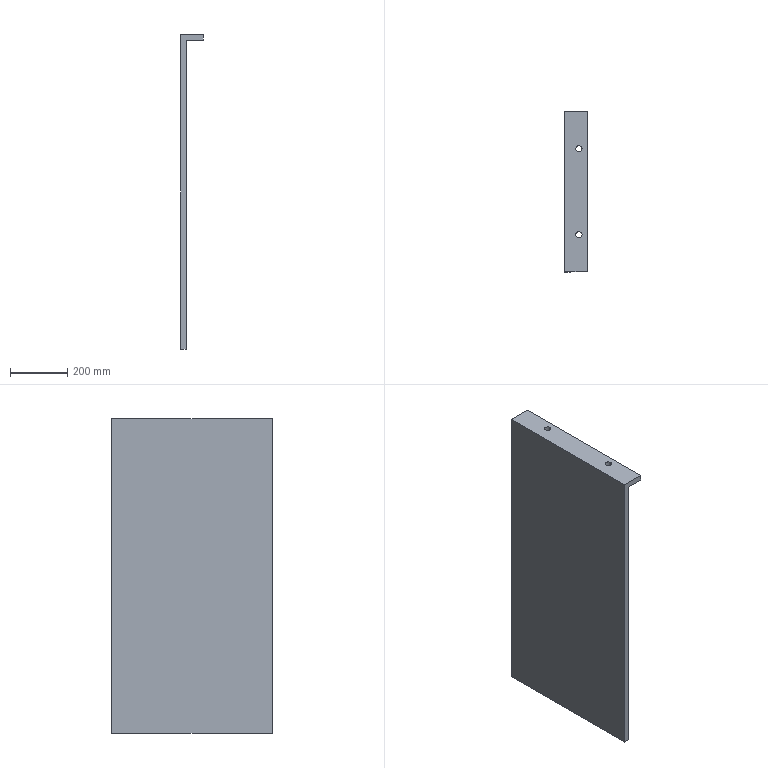Part | SolidWorks | features ICE 3, Extrusion 1 | 1 solid | 12 faces | box 80 x 560 x 1100 mm | volume 12976795 mm3 | plane 8 | cylinder 4 | commonest cylinder face diameters 22 x4
STEP:
#1=CARTESIAN_POINT('',(376.,450.,1100.));
#2=VERTEX_POINT('',#1);
#3=CARTESIAN_POINT('',(354.,450.,1100.));
#4=VERTEX_POINT('',#3);
#5=CARTESIAN_POINT('',(365.,450.,1100.));
#6=DIRECTION('',(0.,0.,-1.));
#7=DIRECTION('',(-1.,0.,0.));
#8=AXIS2_PLACEMENT_3D('',#5,#6,#7);
#9=CIRCLE('',#8,11.);
#10=EDGE_CURVE('',#2,#4,#9,.T.);
#11=ORIENTED_EDGE('',*,*,#10,.F.);
#12=CARTESIAN_POINT('',(376.,450.,1080.));
#13=VERTEX_POINT('',#12);
#14=CARTESIAN_POINT('',(376.,450.,1100.));
#15=DIRECTION('',(0.,0.,-1.));
#16=VECTOR('',#15,1000.);
#17=LINE('',#14,#16);
#18=EDGE_CURVE('',#2,#13,#17,.T.);
#19=ORIENTED_EDGE('',*,*,#18,.T.);
#20=CARTESIAN_POINT('',(354.,450.,1080.));
#21=VERTEX_POINT('',#20);
#22=CARTESIAN_POINT('',(365.,450.,1080.));
#23=DIRECTION('',(0.,0.,-1.));
#24=DIRECTION('',(-1.,0.,0.));
#25=AXIS2_PLACEMENT_3D('',#22,#23,#24);
#26=CIRCLE('',#25,11.);
#27=EDGE_CURVE('',#13,#21,#26,.T.);
#28=ORIENTED_EDGE('',*,*,#27,.T.);
#29=CARTESIAN_POINT('',(354.,450.,1100.));
#30=DIRECTION('',(0.,0.,-1.));
#31=VECTOR('',#30,1000.);
#32=LINE('',#29,#31);
#33=EDGE_CURVE('',#4,#21,#32,.T.);
#34=ORIENTED_EDGE('',*,*,#33,.F.);
#35=EDGE_LOOP('',(#11,#19,#28,#34));
#36=FACE_OUTER_BOUND('',#35,.T.);
#37=CARTESIAN_POINT('',(365.,450.,1100.));
#38=DIRECTION('',(0.,0.,-1.));
#39=DIRECTION('',(-1.,0.,0.));
#40=AXIS2_PLACEMENT_3D('',#37,#38,#39);
#41=CYLINDRICAL_SURFACE('',#40,11.);
#42=ADVANCED_FACE('',(#36),#41,.F.);
#43=CARTESIAN_POINT('',(376.,150.,1100.));
#44=VERTEX_POINT('',#43);
#45=CARTESIAN_POINT('',(354.,150.,1100.));
#46=VERTEX_POINT('',#45);
#47=CARTESIAN_POINT('',(365.,150.,1100.));
#48=DIRECTION('',(0.,0.,-1.));
#49=DIRECTION('',(-1.,0.,0.));
#50=AXIS2_PLACEMENT_3D('',#47,#48,#49);
#51=CIRCLE('',#50,11.);
#52=EDGE_CURVE('',#44,#46,#51,.T.);
#53=ORIENTED_EDGE('',*,*,#52,.F.);
#54=CARTESIAN_POINT('',(376.,150.,1080.));
#55=VERTEX_POINT('',#54);
#56=CARTESIAN_POINT('',(376.,150.,1100.));
#57=DIRECTION('',(0.,0.,-1.));
#58=VECTOR('',#57,1000.);
#59=LINE('',#56,#58);
#60=EDGE_CURVE('',#44,#55,#59,.T.);
#61=ORIENTED_EDGE('',*,*,#60,.T.);
#62=CARTESIAN_POINT('',(354.,150.,1080.));
#63=VERTEX_POINT('',#62);
#64=CARTESIAN_POINT('',(365.,150.,1080.));
#65=DIRECTION('',(0.,0.,-1.));
#66=DIRECTION('',(-1.,0.,0.));
#67=AXIS2_PLACEMENT_3D('',#64,#65,#66);
#68=CIRCLE('',#67,11.);
#69=EDGE_CURVE('',#55,#63,#68,.T.);
#70=ORIENTED_EDGE('',*,*,#69,.T.);
#71=CARTESIAN_POINT('',(354.,150.,1100.));
#72=DIRECTION('',(0.,0.,-1.));
#73=VECTOR('',#72,1000.);
#74=LINE('',#71,#73);
#75=EDGE_CURVE('',#46,#63,#74,.T.);
#76=ORIENTED_EDGE('',*,*,#75,.F.);
#77=EDGE_LOOP('',(#53,#61,#70,#76));
#78=FACE_OUTER_BOUND('',#77,.T.);
#79=CARTESIAN_POINT('',(365.,150.,1100.));
#80=DIRECTION('',(0.,0.,-1.));
#81=DIRECTION('',(-1.,0.,0.));
#82=AXIS2_PLACEMENT_3D('',#79,#80,#81);
#83=CYLINDRICAL_SURFACE('',#82,11.);
#84=ADVANCED_FACE('',(#78),#83,.F.);
#85=CARTESIAN_POINT('',(335.,20.,1080.));
#86=VERTEX_POINT('',#85);
#87=CARTESIAN_POINT('',(335.,580.,1080.));
#88=VERTEX_POINT('',#87);
#89=CARTESIAN_POINT('',(335.,580.,1080.));
#90=DIRECTION('',(0.,1.,0.));
#91=VECTOR('',#90,1000.);
#92=LINE('',#89,#91);
#93=EDGE_CURVE('',#86,#88,#92,.T.);
#94=ORIENTED_EDGE('',*,*,#93,.F.);
#95=CARTESIAN_POINT('',(335.,20.,0.));
#96=VERTEX_POINT('',#95);
#97=CARTESIAN_POINT('',(335.,20.,1100.));
#98=DIRECTION('',(0.,0.,-1.));
#99=VECTOR('',#98,1000.);
#100=LINE('',#97,#99);
#101=EDGE_CURVE('',#86,#96,#100,.T.);
#102=ORIENTED_EDGE('',*,*,#101,.T.);
#103=CARTESIAN_POINT('',(335.,580.,0.));
#104=VERTEX_POINT('',#103);
#105=CARTESIAN_POINT('',(335.,20.,0.));
#106=DIRECTION('',(0.,1.,0.));
#107=VECTOR('',#106,1000.);
#108=LINE('',#105,#107);
#109=EDGE_CURVE('',#96,#104,#108,.T.);
#110=ORIENTED_EDGE('',*,*,#109,.T.);
#111=CARTESIAN_POINT('',(335.,580.,1100.));
#112=DIRECTION('',(0.,0.,-1.));
#113=VECTOR('',#112,1000.);
#114=LINE('',#111,#113);
#115=EDGE_CURVE('',#88,#104,#114,.T.);
#116=ORIENTED_EDGE('',*,*,#115,.F.);
#117=EDGE_LOOP('',(#94,#102,#110,#116));
#118=FACE_OUTER_BOUND('',#117,.T.);
#119=CARTESIAN_POINT('',(335.,20.,1100.));
#120=DIRECTION('',(-1.,0.,0.));
#121=DIRECTION('',(0.,-1.,0.));
#122=AXIS2_PLACEMENT_3D('',#119,#120,#121);
#123=PLANE('',#122);
#124=ADVANCED_FACE('',(#118),#123,.F.);
#125=CARTESIAN_POINT('',(315.,580.,0.));
#126=VERTEX_POINT('',#125);
#127=CARTESIAN_POINT('',(335.,580.,0.));
#128=DIRECTION('',(-1.,0.,0.));
#129=VECTOR('',#128,1000.);
#130=LINE('',#127,#129);
#131=EDGE_CURVE('',#104,#126,#130,.T.);
#132=ORIENTED_EDGE('',*,*,#131,.T.);
#133=CARTESIAN_POINT('',(315.,580.,1100.));
#134=VERTEX_POINT('',#133);
#135=CARTESIAN_POINT('',(315.,580.,1100.));
#136=DIRECTION('',(0.,0.,-1.));
#137=VECTOR('',#136,1000.);
#138=LINE('',#135,#137);
#139=EDGE_CURVE('',#134,#126,#138,.T.);
#140=ORIENTED_EDGE('',*,*,#139,.F.);
#141=CARTESIAN_POINT('',(395.,580.,1100.));
#142=VERTEX_POINT('',#141);
#143=CARTESIAN_POINT('',(335.,580.,1100.));
#144=DIRECTION('',(-1.,0.,0.));
#145=VECTOR('',#144,1000.);
#146=LINE('',#143,#145);
#147=EDGE_CURVE('',#142,#134,#146,.T.);
#148=ORIENTED_EDGE('',*,*,#147,.F.);
#149=CARTESIAN_POINT('',(395.,580.,1080.));
#150=VERTEX_POINT('',#149);
#151=CARTESIAN_POINT('',(395.,580.,1100.));
#152=DIRECTION('',(0.,0.,1.));
#153=VECTOR('',#152,1000.);
#154=LINE('',#151,#153);
#155=EDGE_CURVE('',#150,#142,#154,.T.);
#156=ORIENTED_EDGE('',*,*,#155,.F.);
#157=CARTESIAN_POINT('',(395.,580.,1080.));
#158=DIRECTION('',(-1.,0.,0.));
#159=VECTOR('',#158,1000.);
#160=LINE('',#157,#159);
#161=EDGE_CURVE('',#150,#88,#160,.T.);
#162=ORIENTED_EDGE('',*,*,#161,.T.);
#163=ORIENTED_EDGE('',*,*,#115,.T.);
#164=EDGE_LOOP('',(#132,#140,#148,#156,#162,#163));
#165=FACE_OUTER_BOUND('',#164,.T.);
#166=CARTESIAN_POINT('',(335.,580.,1100.));
#167=DIRECTION('',(0.,-1.,0.));
#168=DIRECTION('',(0.,0.,-1.));
#169=AXIS2_PLACEMENT_3D('',#166,#167,#168);
#170=PLANE('',#169);
#171=ADVANCED_FACE('',(#165),#170,.F.);
#172=CARTESIAN_POINT('',(315.,20.,0.));
#173=VERTEX_POINT('',#172);
#174=CARTESIAN_POINT('',(315.,580.,0.));
#175=DIRECTION('',(0.,-1.,0.));
#176=VECTOR('',#175,1000.);
#177=LINE('',#174,#176);
#178=EDGE_CURVE('',#126,#173,#177,.T.);
#179=ORIENTED_EDGE('',*,*,#178,.T.);
#180=CARTESIAN_POINT('',(315.,20.,1100.));
#181=VERTEX_POINT('',#180);
#182=CARTESIAN_POINT('',(315.,20.,1100.));
#183=DIRECTION('',(0.,0.,-1.));
#184=VECTOR('',#183,1000.);
#185=LINE('',#182,#184);
#186=EDGE_CURVE('',#181,#173,#185,.T.);
#187=ORIENTED_EDGE('',*,*,#186,.F.);
#188=CARTESIAN_POINT('',(315.,580.,1100.));
#189=DIRECTION('',(0.,-1.,0.));
#190=VECTOR('',#189,1000.);
#191=LINE('',#188,#190);
#192=EDGE_CURVE('',#134,#181,#191,.T.);
#193=ORIENTED_EDGE('',*,*,#192,.F.);
#194=ORIENTED_EDGE('',*,*,#139,.T.);
#195=EDGE_LOOP('',(#179,#187,#193,#194));
#196=FACE_OUTER_BOUND('',#195,.T.);
#197=CARTESIAN_POINT('',(315.,580.,1100.));
#198=DIRECTION('',(1.,0.,0.));
#199=DIRECTION('',(0.,1.,0.));
#200=AXIS2_PLACEMENT_3D('',#197,#198,#199);
#201=PLANE('',#200);
#202=ADVANCED_FACE('',(#196),#201,.F.);
#203=CARTESIAN_POINT('',(365.,450.,1100.));
#204=DIRECTION('',(0.,0.,-1.));
#205=DIRECTION('',(-1.,0.,0.));
#206=AXIS2_PLACEMENT_3D('',#203,#204,#205);
#207=CIRCLE('',#206,11.);
#208=EDGE_CURVE('',#4,#2,#207,.T.);
#209=ORIENTED_EDGE('',*,*,#208,.T.);
#210=ORIENTED_EDGE('',*,*,#10,.T.);
#211=EDGE_LOOP('',(#209,#210));
#212=FACE_BOUND('',#211,.T.);
#213=CARTESIAN_POINT('',(365.,150.,1100.));
#214=DIRECTION('',(0.,0.,-1.));
#215=DIRECTION('',(-1.,0.,0.));
#216=AXIS2_PLACEMENT_3D('',#213,#214,#215);
#217=CIRCLE('',#216,11.);
#218=EDGE_CURVE('',#46,#44,#217,.T.);
#219=ORIENTED_EDGE('',*,*,#218,.T.);
#220=ORIENTED_EDGE('',*,*,#52,.T.);
#221=EDGE_LOOP('',(#219,#220));
#222=FACE_BOUND('',#221,.T.);
#223=CARTESIAN_POINT('',(395.,20.,1100.));
#224=VERTEX_POINT('',#223);
#225=CARTESIAN_POINT('',(360.,20.,1100.));
#226=DIRECTION('',(1.,0.,0.));
#227=VECTOR('',#226,1000.);
#228=LINE('',#225,#227);
#229=EDGE_CURVE('',#181,#224,#228,.T.);
#230=ORIENTED_EDGE('',*,*,#229,.T.);
#231=CARTESIAN_POINT('',(395.,580.,1100.));
#232=DIRECTION('',(0.,-1.,0.));
#233=VECTOR('',#232,1000.);
#234=LINE('',#231,#233);
#235=EDGE_CURVE('',#142,#224,#234,.T.);
#236=ORIENTED_EDGE('',*,*,#235,.F.);
#237=ORIENTED_EDGE('',*,*,#147,.T.);
#238=ORIENTED_EDGE('',*,*,#192,.T.);
#239=EDGE_LOOP('',(#230,#236,#237,#238));
#240=FACE_OUTER_BOUND('',#239,.T.);
#241=CARTESIAN_POINT('',(0.,0.,1100.));
#242=DIRECTION('',(0.,0.,1.));
#243=DIRECTION('',(1.,0.,0.));
#244=AXIS2_PLACEMENT_3D('',#241,#242,#243);
#245=PLANE('',#244);
#246=ADVANCED_FACE('',(#212,#222,#240),#245,.T.);
#247=ORIENTED_EDGE('',*,*,#109,.F.);
#248=CARTESIAN_POINT('',(0.,20.,0.));
#249=DIRECTION('',(-1.,0.,0.));
#250=VECTOR('',#249,1000.);
#251=LINE('',#248,#250);
#252=EDGE_CURVE('',#96,#173,#251,.T.);
#253=ORIENTED_EDGE('',*,*,#252,.T.);
#254=ORIENTED_EDGE('',*,*,#178,.F.);
#255=ORIENTED_EDGE('',*,*,#131,.F.);
#256=EDGE_LOOP('',(#247,#253,#254,#255));
#257=FACE_OUTER_BOUND('',#256,.T.);
#258=CARTESIAN_POINT('',(0.,0.,0.));
#259=DIRECTION('',(0.,0.,1.));
#260=DIRECTION('',(1.,0.,0.));
#261=AXIS2_PLACEMENT_3D('',#258,#259,#260);
#262=PLANE('',#261);
#263=ADVANCED_FACE('',(#257),#262,.F.);
#264=ORIENTED_EDGE('',*,*,#252,.F.);
#265=ORIENTED_EDGE('',*,*,#101,.F.);
#266=CARTESIAN_POINT('',(395.,20.,1080.));
#267=VERTEX_POINT('',#266);
#268=CARTESIAN_POINT('',(395.,20.,1080.));
#269=DIRECTION('',(-1.,0.,0.));
#270=VECTOR('',#269,1000.);
#271=LINE('',#268,#270);
#272=EDGE_CURVE('',#267,#86,#271,.T.);
#273=ORIENTED_EDGE('',*,*,#272,.F.);
#274=CARTESIAN_POINT('',(395.,20.,1100.));
#275=DIRECTION('',(0.,0.,-1.));
#276=VECTOR('',#275,1000.);
#277=LINE('',#274,#276);
#278=EDGE_CURVE('',#224,#267,#277,.T.);
#279=ORIENTED_EDGE('',*,*,#278,.F.);
#280=ORIENTED_EDGE('',*,*,#229,.F.);
#281=ORIENTED_EDGE('',*,*,#186,.T.);
#282=EDGE_LOOP('',(#264,#265,#273,#279,#280,#281));
#283=FACE_OUTER_BOUND('',#282,.T.);
#284=CARTESIAN_POINT('',(360.,20.,1100.));
#285=DIRECTION('',(0.,1.,0.));
#286=DIRECTION('',(-1.,0.,0.));
#287=AXIS2_PLACEMENT_3D('',#284,#285,#286);
#288=PLANE('',#287);
#289=ADVANCED_FACE('',(#283),#288,.F.);
#290=CARTESIAN_POINT('',(365.,450.,1080.));
#291=DIRECTION('',(0.,0.,-1.));
#292=DIRECTION('',(-1.,0.,0.));
#293=AXIS2_PLACEMENT_3D('',#290,#291,#292);
#294=CIRCLE('',#293,11.);
#295=EDGE_CURVE('',#21,#13,#294,.T.);
#296=ORIENTED_EDGE('',*,*,#295,.F.);
#297=ORIENTED_EDGE('',*,*,#27,.F.);
#298=EDGE_LOOP('',(#296,#297));
#299=FACE_BOUND('',#298,.T.);
#300=CARTESIAN_POINT('',(365.,150.,1080.));
#301=DIRECTION('',(0.,0.,-1.));
#302=DIRECTION('',(-1.,0.,0.));
#303=AXIS2_PLACEMENT_3D('',#300,#301,#302);
#304=CIRCLE('',#303,11.);
#305=EDGE_CURVE('',#63,#55,#304,.T.);
#306=ORIENTED_EDGE('',*,*,#305,.F.);
#307=ORIENTED_EDGE('',*,*,#69,.F.);
#308=EDGE_LOOP('',(#306,#307));
#309=FACE_BOUND('',#308,.T.);
#310=ORIENTED_EDGE('',*,*,#93,.T.);
#311=ORIENTED_EDGE('',*,*,#161,.F.);
#312=CARTESIAN_POINT('',(395.,580.,1080.));
#313=DIRECTION('',(0.,1.,0.));
#314=VECTOR('',#313,1000.);
#315=LINE('',#312,#314);
#316=EDGE_CURVE('',#267,#150,#315,.T.);
#317=ORIENTED_EDGE('',*,*,#316,.F.);
#318=ORIENTED_EDGE('',*,*,#272,.T.);
#319=EDGE_LOOP('',(#310,#311,#317,#318));
#320=FACE_OUTER_BOUND('',#319,.T.);
#321=CARTESIAN_POINT('',(395.,580.,1080.));
#322=DIRECTION('',(0.,0.,1.));
#323=DIRECTION('',(1.,0.,0.));
#324=AXIS2_PLACEMENT_3D('',#321,#322,#323);
#325=PLANE('',#324);
#326=ADVANCED_FACE('',(#299,#309,#320),#325,.F.);
#327=ORIENTED_EDGE('',*,*,#235,.T.);
#328=ORIENTED_EDGE('',*,*,#278,.T.);
#329=ORIENTED_EDGE('',*,*,#316,.T.);
#330=ORIENTED_EDGE('',*,*,#155,.T.);
#331=EDGE_LOOP('',(#327,#328,#329,#330));
#332=FACE_OUTER_BOUND('',#331,.T.);
#333=CARTESIAN_POINT('',(395.,0.,0.));
#334=DIRECTION('',(1.,0.,0.));
#335=DIRECTION('',(0.,1.,0.));
#336=AXIS2_PLACEMENT_3D('',#333,#334,#335);
#337=PLANE('',#336);
#338=ADVANCED_FACE('',(#332),#337,.T.);
#339=ORIENTED_EDGE('',*,*,#60,.F.);
#340=ORIENTED_EDGE('',*,*,#218,.F.);
#341=ORIENTED_EDGE('',*,*,#75,.T.);
#342=ORIENTED_EDGE('',*,*,#305,.T.);
#343=EDGE_LOOP('',(#339,#340,#341,#342));
#344=FACE_OUTER_BOUND('',#343,.T.);
#345=CARTESIAN_POINT('',(365.,150.,1100.));
#346=DIRECTION('',(0.,0.,-1.));
#347=DIRECTION('',(-1.,0.,0.));
#348=AXIS2_PLACEMENT_3D('',#345,#346,#347);
#349=CYLINDRICAL_SURFACE('',#348,11.);
#350=ADVANCED_FACE('',(#344),#349,.F.);
#351=ORIENTED_EDGE('',*,*,#18,.F.);
#352=ORIENTED_EDGE('',*,*,#208,.F.);
#353=ORIENTED_EDGE('',*,*,#33,.T.);
#354=ORIENTED_EDGE('',*,*,#295,.T.);
#355=EDGE_LOOP('',(#351,#352,#353,#354));
#356=FACE_OUTER_BOUND('',#355,.T.);
#357=CARTESIAN_POINT('',(365.,450.,1100.));
#358=DIRECTION('',(0.,0.,-1.));
#359=DIRECTION('',(-1.,0.,0.));
#360=AXIS2_PLACEMENT_3D('',#357,#358,#359);
#361=CYLINDRICAL_SURFACE('',#360,11.);
#362=ADVANCED_FACE('',(#356),#361,.F.);
#363=CLOSED_SHELL('',(#42,#84,#124,#171,#202,#246,#263,#289,#326,#338,#350,#362));
#364=MANIFOLD_SOLID_BREP('',#363);
#365=CARTESIAN_POINT('',(0.,0.,0.));
#366=DIRECTION('',(0.,0.,1.));
#367=DIRECTION('',(1.,0.,0.));
#368=AXIS2_PLACEMENT_3D('',#365,#366,#367);
#369=(LENGTH_UNIT()NAMED_UNIT(*)SI_UNIT(.MILLI.,.METRE.));
#370=UNCERTAINTY_MEASURE_WITH_UNIT(LENGTH_MEASURE(0.00001),#369,'','');
#371=(NAMED_UNIT(*)PLANE_ANGLE_UNIT()SI_UNIT($,.RADIAN.));
#372=(NAMED_UNIT(*)SI_UNIT($,.STERADIAN.)SOLID_ANGLE_UNIT());
#373=(GEOMETRIC_REPRESENTATION_CONTEXT(3)GLOBAL_UNCERTAINTY_ASSIGNED_CONTEXT((#370))GLOBAL_UNIT_ASSIGNED_CONTEXT((#369,#371,#372))REPRESENTATION_CONTEXT('',''));
#374=ADVANCED_BREP_SHAPE_REPRESENTATION('',(#364,#368),#373);